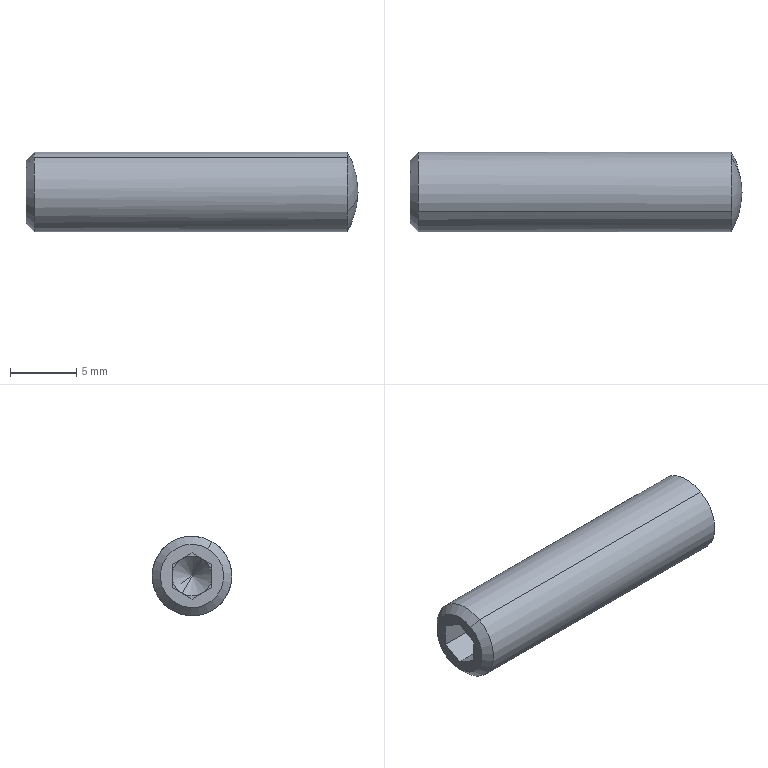Part | STEP file | SANBN6-25-Part-1-6 | 1 solid | 21 faces | box 25 x 6 x 6 mm | volume 665.544 mm3 | plane 13 | cone 4 | sphere 2 | cylinder 2 | commonest cylinder face diameters 6 x2
STEP:
#1=CARTESIAN_POINT('',(8.5,0.,0.));
#2=VERTEX_POINT('',#1);
#3=CARTESIAN_POINT('',(7.,-0.75,1.299));
#4=VERTEX_POINT('',#3);
#5=CARTESIAN_POINT('',(7.,-0.75,1.299));
#6=DIRECTION('',(-0.7071,-0.3536,0.6124));
#7=VECTOR('',#6,1000.);
#8=LINE('',#5,#7);
#9=EDGE_CURVE('',#2,#4,#8,.T.);
#10=ORIENTED_EDGE('',*,*,#9,.F.);
#11=CARTESIAN_POINT('',(7.,0.75,-1.299));
#12=VERTEX_POINT('',#11);
#13=CARTESIAN_POINT('',(7.,0.75,-1.299));
#14=DIRECTION('',(-0.7071,0.3536,-0.6124));
#15=VECTOR('',#14,1000.);
#16=LINE('',#13,#15);
#17=EDGE_CURVE('',#2,#12,#16,.T.);
#18=ORIENTED_EDGE('',*,*,#17,.T.);
#19=CARTESIAN_POINT('',(7.,-0.75,-1.299));
#20=VERTEX_POINT('',#19);
#21=CARTESIAN_POINT('',(7.,0.,0.));
#22=DIRECTION('',(-1.,0.,0.));
#23=DIRECTION('',(0.,0.5,-0.866));
#24=AXIS2_PLACEMENT_3D('',#21,#22,#23);
#25=CIRCLE('',#24,1.5);
#26=EDGE_CURVE('',#12,#20,#25,.T.);
#27=ORIENTED_EDGE('',*,*,#26,.T.);
#28=CARTESIAN_POINT('',(7.,-1.5,0.));
#29=VERTEX_POINT('',#28);
#30=CARTESIAN_POINT('',(7.,0.,0.));
#31=DIRECTION('',(-1.,0.,0.));
#32=DIRECTION('',(0.,0.5,-0.866));
#33=AXIS2_PLACEMENT_3D('',#30,#31,#32);
#34=CIRCLE('',#33,1.5);
#35=EDGE_CURVE('',#20,#29,#34,.T.);
#36=ORIENTED_EDGE('',*,*,#35,.T.);
#37=CARTESIAN_POINT('',(7.,0.,0.));
#38=DIRECTION('',(-1.,0.,0.));
#39=DIRECTION('',(0.,0.5,-0.866));
#40=AXIS2_PLACEMENT_3D('',#37,#38,#39);
#41=CIRCLE('',#40,1.5);
#42=EDGE_CURVE('',#29,#4,#41,.T.);
#43=ORIENTED_EDGE('',*,*,#42,.T.);
#44=EDGE_LOOP('',(#10,#18,#27,#36,#43));
#45=FACE_OUTER_BOUND('',#44,.T.);
#46=CARTESIAN_POINT('',(7.,0.,0.));
#47=DIRECTION('',(-1.,0.,0.));
#48=DIRECTION('',(0.,-0.5,0.866));
#49=AXIS2_PLACEMENT_3D('',#46,#47,#48);
#50=CONICAL_SURFACE('',#49,1.5,0.7854);
#51=ADVANCED_FACE('',(#45),#50,.F.);
#52=CARTESIAN_POINT('',(28.196,-1.5,2.598));
#53=VERTEX_POINT('',#52);
#54=CARTESIAN_POINT('',(28.196,-2.598,-1.5));
#55=VERTEX_POINT('',#54);
#56=CARTESIAN_POINT('',(28.196,0.,0.));
#57=DIRECTION('',(1.,0.,0.));
#58=DIRECTION('',(0.,0.5,-0.866));
#59=AXIS2_PLACEMENT_3D('',#56,#57,#58);
#60=CIRCLE('',#59,3.);
#61=EDGE_CURVE('',#53,#55,#60,.T.);
#62=ORIENTED_EDGE('',*,*,#61,.T.);
#63=CARTESIAN_POINT('',(29.,0.,0.));
#64=VERTEX_POINT('',#63);
#65=CARTESIAN_POINT('',(23.,0.,0.));
#66=DIRECTION('',(0.,-0.5,0.866));
#67=DIRECTION('',(0.,-0.866,-0.5));
#68=AXIS2_PLACEMENT_3D('',#65,#66,#67);
#69=CIRCLE('',#68,6.);
#70=EDGE_CURVE('',#55,#64,#69,.T.);
#71=ORIENTED_EDGE('',*,*,#70,.T.);
#72=CARTESIAN_POINT('',(28.196,2.598,1.5));
#73=VERTEX_POINT('',#72);
#74=CARTESIAN_POINT('',(23.,0.,0.));
#75=DIRECTION('',(0.,0.5,-0.866));
#76=DIRECTION('',(0.,0.866,0.5));
#77=AXIS2_PLACEMENT_3D('',#74,#75,#76);
#78=CIRCLE('',#77,6.);
#79=EDGE_CURVE('',#73,#64,#78,.T.);
#80=ORIENTED_EDGE('',*,*,#79,.F.);
#81=CARTESIAN_POINT('',(28.196,0.,0.));
#82=DIRECTION('',(1.,0.,0.));
#83=DIRECTION('',(0.,0.5,-0.866));
#84=AXIS2_PLACEMENT_3D('',#81,#82,#83);
#85=CIRCLE('',#84,3.);
#86=EDGE_CURVE('',#73,#53,#85,.T.);
#87=ORIENTED_EDGE('',*,*,#86,.T.);
#88=EDGE_LOOP('',(#62,#71,#80,#87));
#89=FACE_OUTER_BOUND('',#88,.T.);
#90=CARTESIAN_POINT('',(23.,0.,0.));
#91=DIRECTION('',(0.,-0.5,0.866));
#92=DIRECTION('',(0.,0.866,0.5));
#93=AXIS2_PLACEMENT_3D('',#90,#91,#92);
#94=SPHERICAL_SURFACE('',#93,6.);
#95=ADVANCED_FACE('',(#89),#94,.T.);
#96=CARTESIAN_POINT('',(4.614,1.5,-2.598));
#97=VERTEX_POINT('',#96);
#98=CARTESIAN_POINT('',(4.614,-1.5,2.598));
#99=VERTEX_POINT('',#98);
#100=CARTESIAN_POINT('',(4.614,0.,0.));
#101=DIRECTION('',(1.,0.,0.));
#102=DIRECTION('',(0.,0.5,-0.866));
#103=AXIS2_PLACEMENT_3D('',#100,#101,#102);
#104=CIRCLE('',#103,3.);
#105=EDGE_CURVE('',#97,#99,#104,.T.);
#106=ORIENTED_EDGE('',*,*,#105,.T.);
#107=CARTESIAN_POINT('',(29.,-1.5,2.598));
#108=DIRECTION('',(1.,0.,0.));
#109=VECTOR('',#108,1000.);
#110=LINE('',#107,#109);
#111=EDGE_CURVE('',#99,#53,#110,.T.);
#112=ORIENTED_EDGE('',*,*,#111,.T.);
#113=ORIENTED_EDGE('',*,*,#86,.F.);
#114=CARTESIAN_POINT('',(28.196,1.5,-2.598));
#115=VERTEX_POINT('',#114);
#116=CARTESIAN_POINT('',(28.196,0.,0.));
#117=DIRECTION('',(1.,0.,0.));
#118=DIRECTION('',(0.,0.5,-0.866));
#119=AXIS2_PLACEMENT_3D('',#116,#117,#118);
#120=CIRCLE('',#119,3.);
#121=EDGE_CURVE('',#115,#73,#120,.T.);
#122=ORIENTED_EDGE('',*,*,#121,.F.);
#123=CARTESIAN_POINT('',(29.,1.5,-2.598));
#124=DIRECTION('',(1.,0.,0.));
#125=VECTOR('',#124,1000.);
#126=LINE('',#123,#125);
#127=EDGE_CURVE('',#97,#115,#126,.T.);
#128=ORIENTED_EDGE('',*,*,#127,.F.);
#129=EDGE_LOOP('',(#106,#112,#113,#122,#128));
#130=FACE_OUTER_BOUND('',#129,.T.);
#131=CARTESIAN_POINT('',(29.,0.,0.));
#132=DIRECTION('',(1.,0.,0.));
#133=DIRECTION('',(0.,0.5,-0.866));
#134=AXIS2_PLACEMENT_3D('',#131,#132,#133);
#135=CYLINDRICAL_SURFACE('',#134,3.);
#136=ADVANCED_FACE('',(#130),#135,.T.);
#137=CARTESIAN_POINT('',(4.,1.193,-2.067));
#138=VERTEX_POINT('',#137);
#139=CARTESIAN_POINT('',(4.,-1.193,2.067));
#140=VERTEX_POINT('',#139);
#141=CARTESIAN_POINT('',(4.,0.,0.));
#142=DIRECTION('',(1.,0.,0.));
#143=DIRECTION('',(0.,0.5,-0.866));
#144=AXIS2_PLACEMENT_3D('',#141,#142,#143);
#145=CIRCLE('',#144,2.387);
#146=EDGE_CURVE('',#138,#140,#145,.T.);
#147=ORIENTED_EDGE('',*,*,#146,.T.);
#148=CARTESIAN_POINT('',(4.,-1.193,2.067));
#149=DIRECTION('',(0.7071,-0.3536,0.6124));
#150=VECTOR('',#149,1000.);
#151=LINE('',#148,#150);
#152=EDGE_CURVE('',#140,#99,#151,.T.);
#153=ORIENTED_EDGE('',*,*,#152,.T.);
#154=ORIENTED_EDGE('',*,*,#105,.F.);
#155=CARTESIAN_POINT('',(4.,1.193,-2.067));
#156=DIRECTION('',(0.7071,0.3536,-0.6124));
#157=VECTOR('',#156,1000.);
#158=LINE('',#155,#157);
#159=EDGE_CURVE('',#138,#97,#158,.T.);
#160=ORIENTED_EDGE('',*,*,#159,.F.);
#161=EDGE_LOOP('',(#147,#153,#154,#160));
#162=FACE_OUTER_BOUND('',#161,.T.);
#163=CARTESIAN_POINT('',(4.,0.,0.));
#164=DIRECTION('',(1.,0.,0.));
#165=DIRECTION('',(0.,0.5,-0.866));
#166=AXIS2_PLACEMENT_3D('',#163,#164,#165);
#167=CONICAL_SURFACE('',#166,2.387,0.7854);
#168=ADVANCED_FACE('',(#162),#167,.T.);
#169=ORIENTED_EDGE('',*,*,#35,.F.);
#170=CARTESIAN_POINT('',(7.,-1.5,-0.866));
#171=VERTEX_POINT('',#170);
#172=CARTESIAN_POINT('',(7.,-1.5,-0.866));
#173=DIRECTION('',(0.,0.866,-0.5));
#174=VECTOR('',#173,1000.);
#175=LINE('',#172,#174);
#176=EDGE_CURVE('',#171,#20,#175,.T.);
#177=ORIENTED_EDGE('',*,*,#176,.F.);
#178=CARTESIAN_POINT('',(7.,-1.5,0.866));
#179=DIRECTION('',(0.,0.,-1.));
#180=VECTOR('',#179,1000.);
#181=LINE('',#178,#180);
#182=EDGE_CURVE('',#29,#171,#181,.T.);
#183=ORIENTED_EDGE('',*,*,#182,.F.);
#184=EDGE_LOOP('',(#169,#177,#183));
#185=FACE_OUTER_BOUND('',#184,.T.);
#186=CARTESIAN_POINT('',(7.,0.,0.));
#187=DIRECTION('',(1.,0.,0.));
#188=DIRECTION('',(0.,0.5,-0.866));
#189=AXIS2_PLACEMENT_3D('',#186,#187,#188);
#190=PLANE('',#189);
#191=ADVANCED_FACE('',(#185),#190,.F.);
#192=ORIENTED_EDGE('',*,*,#42,.F.);
#193=CARTESIAN_POINT('',(7.,-1.5,0.866));
#194=VERTEX_POINT('',#193);
#195=CARTESIAN_POINT('',(7.,-1.5,0.866));
#196=DIRECTION('',(0.,0.,-1.));
#197=VECTOR('',#196,1000.);
#198=LINE('',#195,#197);
#199=EDGE_CURVE('',#194,#29,#198,.T.);
#200=ORIENTED_EDGE('',*,*,#199,.F.);
#201=CARTESIAN_POINT('',(7.,0.,1.732));
#202=DIRECTION('',(0.,-0.866,-0.5));
#203=VECTOR('',#202,1000.);
#204=LINE('',#201,#203);
#205=EDGE_CURVE('',#4,#194,#204,.T.);
#206=ORIENTED_EDGE('',*,*,#205,.F.);
#207=EDGE_LOOP('',(#192,#200,#206));
#208=FACE_OUTER_BOUND('',#207,.T.);
#209=CARTESIAN_POINT('',(7.,0.,0.));
#210=DIRECTION('',(1.,0.,0.));
#211=DIRECTION('',(0.,0.5,-0.866));
#212=AXIS2_PLACEMENT_3D('',#209,#210,#211);
#213=PLANE('',#212);
#214=ADVANCED_FACE('',(#208),#213,.F.);
#215=CARTESIAN_POINT('',(7.,0.75,1.299));
#216=VERTEX_POINT('',#215);
#217=CARTESIAN_POINT('',(7.,0.,0.));
#218=DIRECTION('',(-1.,0.,0.));
#219=DIRECTION('',(0.,0.5,-0.866));
#220=AXIS2_PLACEMENT_3D('',#217,#218,#219);
#221=CIRCLE('',#220,1.5);
#222=EDGE_CURVE('',#4,#216,#221,.T.);
#223=ORIENTED_EDGE('',*,*,#222,.F.);
#224=CARTESIAN_POINT('',(7.,0.,1.732));
#225=VERTEX_POINT('',#224);
#226=CARTESIAN_POINT('',(7.,0.,1.732));
#227=DIRECTION('',(0.,-0.866,-0.5));
#228=VECTOR('',#227,1000.);
#229=LINE('',#226,#228);
#230=EDGE_CURVE('',#225,#4,#229,.T.);
#231=ORIENTED_EDGE('',*,*,#230,.F.);
#232=CARTESIAN_POINT('',(7.,1.5,0.866));
#233=DIRECTION('',(0.,-0.866,0.5));
#234=VECTOR('',#233,1000.);
#235=LINE('',#232,#234);
#236=EDGE_CURVE('',#216,#225,#235,.T.);
#237=ORIENTED_EDGE('',*,*,#236,.F.);
#238=EDGE_LOOP('',(#223,#231,#237));
#239=FACE_OUTER_BOUND('',#238,.T.);
#240=CARTESIAN_POINT('',(7.,0.,0.));
#241=DIRECTION('',(1.,0.,0.));
#242=DIRECTION('',(0.,0.5,-0.866));
#243=AXIS2_PLACEMENT_3D('',#240,#241,#242);
#244=PLANE('',#243);
#245=ADVANCED_FACE('',(#239),#244,.F.);
#246=CARTESIAN_POINT('',(7.,1.5,0.));
#247=VERTEX_POINT('',#246);
#248=CARTESIAN_POINT('',(7.,0.,0.));
#249=DIRECTION('',(-1.,0.,0.));
#250=DIRECTION('',(0.,0.5,-0.866));
#251=AXIS2_PLACEMENT_3D('',#248,#249,#250);
#252=CIRCLE('',#251,1.5);
#253=EDGE_CURVE('',#216,#247,#252,.T.);
#254=ORIENTED_EDGE('',*,*,#253,.F.);
#255=CARTESIAN_POINT('',(7.,1.5,0.866));
#256=VERTEX_POINT('',#255);
#257=CARTESIAN_POINT('',(7.,1.5,0.866));
#258=DIRECTION('',(0.,-0.866,0.5));
#259=VECTOR('',#258,1000.);
#260=LINE('',#257,#259);
#261=EDGE_CURVE('',#256,#216,#260,.T.);
#262=ORIENTED_EDGE('',*,*,#261,.F.);
#263=CARTESIAN_POINT('',(7.,1.5,-0.866));
#264=DIRECTION('',(0.,0.,1.));
#265=VECTOR('',#264,1000.);
#266=LINE('',#263,#265);
#267=EDGE_CURVE('',#247,#256,#266,.T.);
#268=ORIENTED_EDGE('',*,*,#267,.F.);
#269=EDGE_LOOP('',(#254,#262,#268));
#270=FACE_OUTER_BOUND('',#269,.T.);
#271=CARTESIAN_POINT('',(7.,0.,0.));
#272=DIRECTION('',(1.,0.,0.));
#273=DIRECTION('',(0.,0.5,-0.866));
#274=AXIS2_PLACEMENT_3D('',#271,#272,#273);
#275=PLANE('',#274);
#276=ADVANCED_FACE('',(#270),#275,.F.);
#277=ORIENTED_EDGE('',*,*,#26,.F.);
#278=CARTESIAN_POINT('',(7.,0.,-1.732));
#279=VERTEX_POINT('',#278);
#280=CARTESIAN_POINT('',(7.,0.,-1.732));
#281=DIRECTION('',(0.,0.866,0.5));
#282=VECTOR('',#281,1000.);
#283=LINE('',#280,#282);
#284=EDGE_CURVE('',#279,#12,#283,.T.);
#285=ORIENTED_EDGE('',*,*,#284,.F.);
#286=CARTESIAN_POINT('',(7.,-1.5,-0.866));
#287=DIRECTION('',(0.,0.866,-0.5));
#288=VECTOR('',#287,1000.);
#289=LINE('',#286,#288);
#290=EDGE_CURVE('',#20,#279,#289,.T.);
#291=ORIENTED_EDGE('',*,*,#290,.F.);
#292=EDGE_LOOP('',(#277,#285,#291));
#293=FACE_OUTER_BOUND('',#292,.T.);
#294=CARTESIAN_POINT('',(7.,0.,0.));
#295=DIRECTION('',(1.,0.,0.));
#296=DIRECTION('',(0.,0.5,-0.866));
#297=AXIS2_PLACEMENT_3D('',#294,#295,#296);
#298=PLANE('',#297);
#299=ADVANCED_FACE('',(#293),#298,.F.);
#300=ORIENTED_EDGE('',*,*,#146,.F.);
#301=CARTESIAN_POINT('',(4.,0.,0.));
#302=DIRECTION('',(1.,0.,0.));
#303=DIRECTION('',(0.,0.5,-0.866));
#304=AXIS2_PLACEMENT_3D('',#301,#302,#303);
#305=CIRCLE('',#304,2.387);
#306=EDGE_CURVE('',#140,#138,#305,.T.);
#307=ORIENTED_EDGE('',*,*,#306,.F.);
#308=EDGE_LOOP('',(#300,#307));
#309=FACE_OUTER_BOUND('',#308,.T.);
#310=CARTESIAN_POINT('',(4.,0.,1.732));
#311=VERTEX_POINT('',#310);
#312=CARTESIAN_POINT('',(4.,-1.5,0.866));
#313=VERTEX_POINT('',#312);
#314=CARTESIAN_POINT('',(4.,0.,1.732));
#315=DIRECTION('',(0.,-0.866,-0.5));
#316=VECTOR('',#315,1000.);
#317=LINE('',#314,#316);
#318=EDGE_CURVE('',#311,#313,#317,.T.);
#319=ORIENTED_EDGE('',*,*,#318,.T.);
#320=CARTESIAN_POINT('',(4.,-1.5,-0.866));
#321=VERTEX_POINT('',#320);
#322=CARTESIAN_POINT('',(4.,-1.5,0.866));
#323=DIRECTION('',(0.,0.,-1.));
#324=VECTOR('',#323,1000.);
#325=LINE('',#322,#324);
#326=EDGE_CURVE('',#313,#321,#325,.T.);
#327=ORIENTED_EDGE('',*,*,#326,.T.);
#328=CARTESIAN_POINT('',(4.,0.,-1.732));
#329=VERTEX_POINT('',#328);
#330=CARTESIAN_POINT('',(4.,-1.5,-0.866));
#331=DIRECTION('',(0.,0.866,-0.5));
#332=VECTOR('',#331,1000.);
#333=LINE('',#330,#332);
#334=EDGE_CURVE('',#321,#329,#333,.T.);
#335=ORIENTED_EDGE('',*,*,#334,.T.);
#336=CARTESIAN_POINT('',(4.,1.5,-0.866));
#337=VERTEX_POINT('',#336);
#338=CARTESIAN_POINT('',(4.,0.,-1.732));
#339=DIRECTION('',(0.,0.866,0.5));
#340=VECTOR('',#339,1000.);
#341=LINE('',#338,#340);
#342=EDGE_CURVE('',#329,#337,#341,.T.);
#343=ORIENTED_EDGE('',*,*,#342,.T.);
#344=CARTESIAN_POINT('',(4.,1.5,0.866));
#345=VERTEX_POINT('',#344);
#346=CARTESIAN_POINT('',(4.,1.5,-0.866));
#347=DIRECTION('',(0.,0.,1.));
#348=VECTOR('',#347,1000.);
#349=LINE('',#346,#348);
#350=EDGE_CURVE('',#337,#345,#349,.T.);
#351=ORIENTED_EDGE('',*,*,#350,.T.);
#352=CARTESIAN_POINT('',(4.,1.5,0.866));
#353=DIRECTION('',(0.,-0.866,0.5));
#354=VECTOR('',#353,1000.);
#355=LINE('',#352,#354);
#356=EDGE_CURVE('',#345,#311,#355,.T.);
#357=ORIENTED_EDGE('',*,*,#356,.T.);
#358=EDGE_LOOP('',(#319,#327,#335,#343,#351,#357));
#359=FACE_BOUND('',#358,.T.);
#360=CARTESIAN_POINT('',(4.,0.,0.));
#361=DIRECTION('',(1.,0.,0.));
#362=DIRECTION('',(0.,0.5,-0.866));
#363=AXIS2_PLACEMENT_3D('',#360,#361,#362);
#364=PLANE('',#363);
#365=ADVANCED_FACE('',(#309,#359),#364,.F.);
#366=ORIENTED_EDGE('',*,*,#152,.F.);
#367=ORIENTED_EDGE('',*,*,#306,.T.);
#368=ORIENTED_EDGE('',*,*,#159,.T.);
#369=CARTESIAN_POINT('',(4.614,0.,0.));
#370=DIRECTION('',(1.,0.,0.));
#371=DIRECTION('',(0.,0.5,-0.866));
#372=AXIS2_PLACEMENT_3D('',#369,#370,#371);
#373=CIRCLE('',#372,3.);
#374=EDGE_CURVE('',#99,#97,#373,.T.);
#375=ORIENTED_EDGE('',*,*,#374,.F.);
#376=EDGE_LOOP('',(#366,#367,#368,#375));
#377=FACE_OUTER_BOUND('',#376,.T.);
#378=CARTESIAN_POINT('',(4.,0.,0.));
#379=DIRECTION('',(1.,0.,0.));
#380=DIRECTION('',(0.,0.5,-0.866));
#381=AXIS2_PLACEMENT_3D('',#378,#379,#380);
#382=CONICAL_SURFACE('',#381,2.387,0.7854);
#383=ADVANCED_FACE('',(#377),#382,.T.);
#384=ORIENTED_EDGE('',*,*,#111,.F.);
#385=ORIENTED_EDGE('',*,*,#374,.T.);
#386=ORIENTED_EDGE('',*,*,#127,.T.);
#387=CARTESIAN_POINT('',(28.196,0.,0.));
#388=DIRECTION('',(1.,0.,0.));
#389=DIRECTION('',(0.,0.5,-0.866));
#390=AXIS2_PLACEMENT_3D('',#387,#388,#389);
#391=CIRCLE('',#390,3.);
#392=EDGE_CURVE('',#55,#115,#391,.T.);
#393=ORIENTED_EDGE('',*,*,#392,.F.);
#394=ORIENTED_EDGE('',*,*,#61,.F.);
#395=EDGE_LOOP('',(#384,#385,#386,#393,#394));
#396=FACE_OUTER_BOUND('',#395,.T.);
#397=CARTESIAN_POINT('',(29.,0.,0.));
#398=DIRECTION('',(1.,0.,0.));
#399=DIRECTION('',(0.,0.5,-0.866));
#400=AXIS2_PLACEMENT_3D('',#397,#398,#399);
#401=CYLINDRICAL_SURFACE('',#400,3.);
#402=ADVANCED_FACE('',(#396),#401,.T.);
#403=ORIENTED_EDGE('',*,*,#70,.F.);
#404=ORIENTED_EDGE('',*,*,#392,.T.);
#405=ORIENTED_EDGE('',*,*,#121,.T.);
#406=ORIENTED_EDGE('',*,*,#79,.T.);
#407=EDGE_LOOP('',(#403,#404,#405,#406));
#408=FACE_OUTER_BOUND('',#407,.T.);
#409=CARTESIAN_POINT('',(23.,0.,0.));
#410=DIRECTION('',(0.,-0.5,0.866));
#411=DIRECTION('',(0.,0.866,0.5));
#412=AXIS2_PLACEMENT_3D('',#409,#410,#411);
#413=SPHERICAL_SURFACE('',#412,6.);
#414=ADVANCED_FACE('',(#408),#413,.T.);
#415=ORIENTED_EDGE('',*,*,#318,.F.);
#416=CARTESIAN_POINT('',(7.,0.,1.732));
#417=DIRECTION('',(-1.,0.,0.));
#418=VECTOR('',#417,1000.);
#419=LINE('',#416,#418);
#420=EDGE_CURVE('',#225,#311,#419,.T.);
#421=ORIENTED_EDGE('',*,*,#420,.F.);
#422=ORIENTED_EDGE('',*,*,#230,.T.);
#423=ORIENTED_EDGE('',*,*,#205,.T.);
#424=CARTESIAN_POINT('',(7.,-1.5,0.866));
#425=DIRECTION('',(-1.,0.,0.));
#426=VECTOR('',#425,1000.);
#427=LINE('',#424,#426);
#428=EDGE_CURVE('',#194,#313,#427,.T.);
#429=ORIENTED_EDGE('',*,*,#428,.T.);
#430=EDGE_LOOP('',(#415,#421,#422,#423,#429));
#431=FACE_OUTER_BOUND('',#430,.T.);
#432=CARTESIAN_POINT('',(7.,0.,1.732));
#433=DIRECTION('',(0.,0.5,-0.866));
#434=DIRECTION('',(-1.,0.,0.));
#435=AXIS2_PLACEMENT_3D('',#432,#433,#434);
#436=PLANE('',#435);
#437=ADVANCED_FACE('',(#431),#436,.T.);
#438=ORIENTED_EDGE('',*,*,#326,.F.);
#439=ORIENTED_EDGE('',*,*,#428,.F.);
#440=ORIENTED_EDGE('',*,*,#199,.T.);
#441=ORIENTED_EDGE('',*,*,#182,.T.);
#442=CARTESIAN_POINT('',(7.,-1.5,-0.866));
#443=DIRECTION('',(-1.,0.,0.));
#444=VECTOR('',#443,1000.);
#445=LINE('',#442,#444);
#446=EDGE_CURVE('',#171,#321,#445,.T.);
#447=ORIENTED_EDGE('',*,*,#446,.T.);
#448=EDGE_LOOP('',(#438,#439,#440,#441,#447));
#449=FACE_OUTER_BOUND('',#448,.T.);
#450=CARTESIAN_POINT('',(7.,-1.5,0.866));
#451=DIRECTION('',(0.,1.,0.));
#452=DIRECTION('',(0.,0.,1.));
#453=AXIS2_PLACEMENT_3D('',#450,#451,#452);
#454=PLANE('',#453);
#455=ADVANCED_FACE('',(#449),#454,.T.);
#456=ORIENTED_EDGE('',*,*,#334,.F.);
#457=ORIENTED_EDGE('',*,*,#446,.F.);
#458=ORIENTED_EDGE('',*,*,#176,.T.);
#459=ORIENTED_EDGE('',*,*,#290,.T.);
#460=CARTESIAN_POINT('',(7.,0.,-1.732));
#461=DIRECTION('',(-1.,0.,0.));
#462=VECTOR('',#461,1000.);
#463=LINE('',#460,#462);
#464=EDGE_CURVE('',#279,#329,#463,.T.);
#465=ORIENTED_EDGE('',*,*,#464,.T.);
#466=EDGE_LOOP('',(#456,#457,#458,#459,#465));
#467=FACE_OUTER_BOUND('',#466,.T.);
#468=CARTESIAN_POINT('',(7.,-1.5,-0.866));
#469=DIRECTION('',(0.,0.5,0.866));
#470=DIRECTION('',(0.,-0.866,0.5));
#471=AXIS2_PLACEMENT_3D('',#468,#469,#470);
#472=PLANE('',#471);
#473=ADVANCED_FACE('',(#467),#472,.T.);
#474=ORIENTED_EDGE('',*,*,#342,.F.);
#475=ORIENTED_EDGE('',*,*,#464,.F.);
#476=ORIENTED_EDGE('',*,*,#284,.T.);
#477=CARTESIAN_POINT('',(7.,1.5,-0.866));
#478=VERTEX_POINT('',#477);
#479=CARTESIAN_POINT('',(7.,0.,-1.732));
#480=DIRECTION('',(0.,0.866,0.5));
#481=VECTOR('',#480,1000.);
#482=LINE('',#479,#481);
#483=EDGE_CURVE('',#12,#478,#482,.T.);
#484=ORIENTED_EDGE('',*,*,#483,.T.);
#485=CARTESIAN_POINT('',(7.,1.5,-0.866));
#486=DIRECTION('',(-1.,0.,0.));
#487=VECTOR('',#486,1000.);
#488=LINE('',#485,#487);
#489=EDGE_CURVE('',#478,#337,#488,.T.);
#490=ORIENTED_EDGE('',*,*,#489,.T.);
#491=EDGE_LOOP('',(#474,#475,#476,#484,#490));
#492=FACE_OUTER_BOUND('',#491,.T.);
#493=CARTESIAN_POINT('',(7.,0.,-1.732));
#494=DIRECTION('',(0.,-0.5,0.866));
#495=DIRECTION('',(1.,0.,0.));
#496=AXIS2_PLACEMENT_3D('',#493,#494,#495);
#497=PLANE('',#496);
#498=ADVANCED_FACE('',(#492),#497,.T.);
#499=ORIENTED_EDGE('',*,*,#350,.F.);
#500=ORIENTED_EDGE('',*,*,#489,.F.);
#501=CARTESIAN_POINT('',(7.,1.5,-0.866));
#502=DIRECTION('',(0.,0.,1.));
#503=VECTOR('',#502,1000.);
#504=LINE('',#501,#503);
#505=EDGE_CURVE('',#478,#247,#504,.T.);
#506=ORIENTED_EDGE('',*,*,#505,.T.);
#507=ORIENTED_EDGE('',*,*,#267,.T.);
#508=CARTESIAN_POINT('',(7.,1.5,0.866));
#509=DIRECTION('',(-1.,0.,0.));
#510=VECTOR('',#509,1000.);
#511=LINE('',#508,#510);
#512=EDGE_CURVE('',#256,#345,#511,.T.);
#513=ORIENTED_EDGE('',*,*,#512,.T.);
#514=EDGE_LOOP('',(#499,#500,#506,#507,#513));
#515=FACE_OUTER_BOUND('',#514,.T.);
#516=CARTESIAN_POINT('',(7.,1.5,-0.866));
#517=DIRECTION('',(0.,-1.,0.));
#518=DIRECTION('',(0.,0.,-1.));
#519=AXIS2_PLACEMENT_3D('',#516,#517,#518);
#520=PLANE('',#519);
#521=ADVANCED_FACE('',(#515),#520,.T.);
#522=ORIENTED_EDGE('',*,*,#356,.F.);
#523=ORIENTED_EDGE('',*,*,#512,.F.);
#524=ORIENTED_EDGE('',*,*,#261,.T.);
#525=ORIENTED_EDGE('',*,*,#236,.T.);
#526=ORIENTED_EDGE('',*,*,#420,.T.);
#527=EDGE_LOOP('',(#522,#523,#524,#525,#526));
#528=FACE_OUTER_BOUND('',#527,.T.);
#529=CARTESIAN_POINT('',(7.,1.5,0.866));
#530=DIRECTION('',(0.,-0.5,-0.866));
#531=DIRECTION('',(0.,0.866,-0.5));
#532=AXIS2_PLACEMENT_3D('',#529,#530,#531);
#533=PLANE('',#532);
#534=ADVANCED_FACE('',(#528),#533,.T.);
#535=CARTESIAN_POINT('',(7.,0.,0.));
#536=DIRECTION('',(-1.,0.,0.));
#537=DIRECTION('',(0.,0.5,-0.866));
#538=AXIS2_PLACEMENT_3D('',#535,#536,#537);
#539=CIRCLE('',#538,1.5);
#540=EDGE_CURVE('',#247,#12,#539,.T.);
#541=ORIENTED_EDGE('',*,*,#540,.F.);
#542=ORIENTED_EDGE('',*,*,#505,.F.);
#543=ORIENTED_EDGE('',*,*,#483,.F.);
#544=EDGE_LOOP('',(#541,#542,#543));
#545=FACE_OUTER_BOUND('',#544,.T.);
#546=CARTESIAN_POINT('',(7.,0.,0.));
#547=DIRECTION('',(1.,0.,0.));
#548=DIRECTION('',(0.,0.5,-0.866));
#549=AXIS2_PLACEMENT_3D('',#546,#547,#548);
#550=PLANE('',#549);
#551=ADVANCED_FACE('',(#545),#550,.F.);
#552=ORIENTED_EDGE('',*,*,#17,.F.);
#553=ORIENTED_EDGE('',*,*,#9,.T.);
#554=ORIENTED_EDGE('',*,*,#222,.T.);
#555=ORIENTED_EDGE('',*,*,#253,.T.);
#556=ORIENTED_EDGE('',*,*,#540,.T.);
#557=EDGE_LOOP('',(#552,#553,#554,#555,#556));
#558=FACE_OUTER_BOUND('',#557,.T.);
#559=CARTESIAN_POINT('',(7.,0.,0.));
#560=DIRECTION('',(-1.,0.,0.));
#561=DIRECTION('',(0.,-0.5,0.866));
#562=AXIS2_PLACEMENT_3D('',#559,#560,#561);
#563=CONICAL_SURFACE('',#562,1.5,0.7854);
#564=ADVANCED_FACE('',(#558),#563,.F.);
#565=CLOSED_SHELL('',(#51,#95,#136,#168,#191,#214,#245,#276,#299,#365,#383,#402,#414,#437,#455,#473,#498,#521,#534,#551,#564));
#566=MANIFOLD_SOLID_BREP('',#565);
#567=CARTESIAN_POINT('',(0.,0.,0.));
#568=DIRECTION('',(0.,0.,1.));
#569=DIRECTION('',(1.,0.,0.));
#570=AXIS2_PLACEMENT_3D('',#567,#568,#569);
#571=(LENGTH_UNIT()NAMED_UNIT(*)SI_UNIT(.MILLI.,.METRE.));
#572=UNCERTAINTY_MEASURE_WITH_UNIT(LENGTH_MEASURE(0.00001),#571,'','');
#573=(NAMED_UNIT(*)PLANE_ANGLE_UNIT()SI_UNIT($,.RADIAN.));
#574=(NAMED_UNIT(*)SI_UNIT($,.STERADIAN.)SOLID_ANGLE_UNIT());
#575=(GEOMETRIC_REPRESENTATION_CONTEXT(3)GLOBAL_UNCERTAINTY_ASSIGNED_CONTEXT((#572))GLOBAL_UNIT_ASSIGNED_CONTEXT((#571,#573,#574))REPRESENTATION_CONTEXT('',''));
#576=ADVANCED_BREP_SHAPE_REPRESENTATION('',(#566,#570),#575);